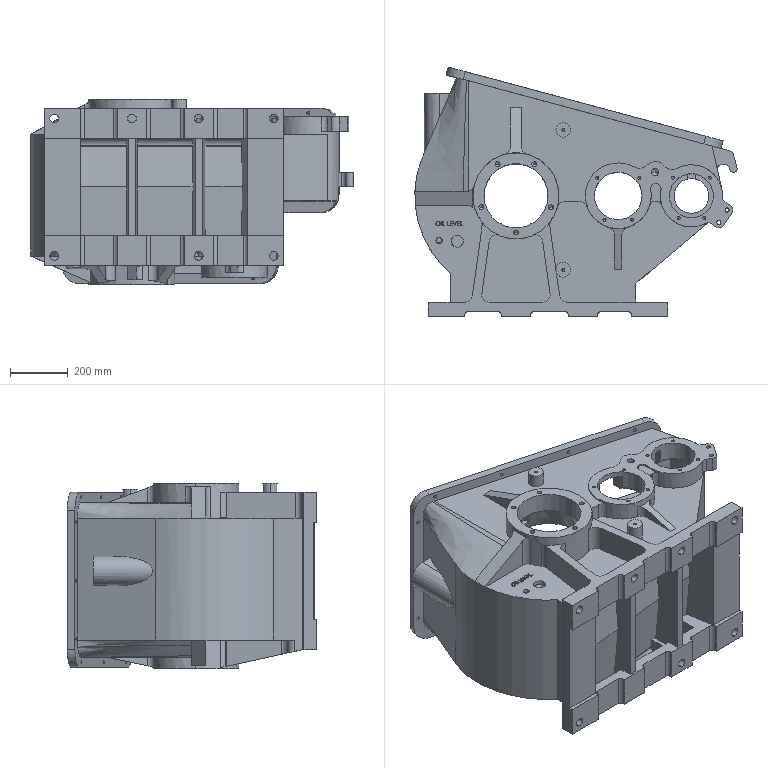Part | SolidWorks | features ICE 78, HoleWzd 17, Fillet 7, 3DProfileFeature 6, RevCut 4, Blend 2, Extrusion 1 | 1 solid | 709 faces | box 1118 x 865.604 x 644.525 mm | volume 64344550 mm3 | plane 329 | cylinder 281 | cone 81 | spline 18 | commonest cylinder face diameters 10.716 x62 50.8 x57 76.2 x23 16.667 x20 25.4 x19 30.163 x14